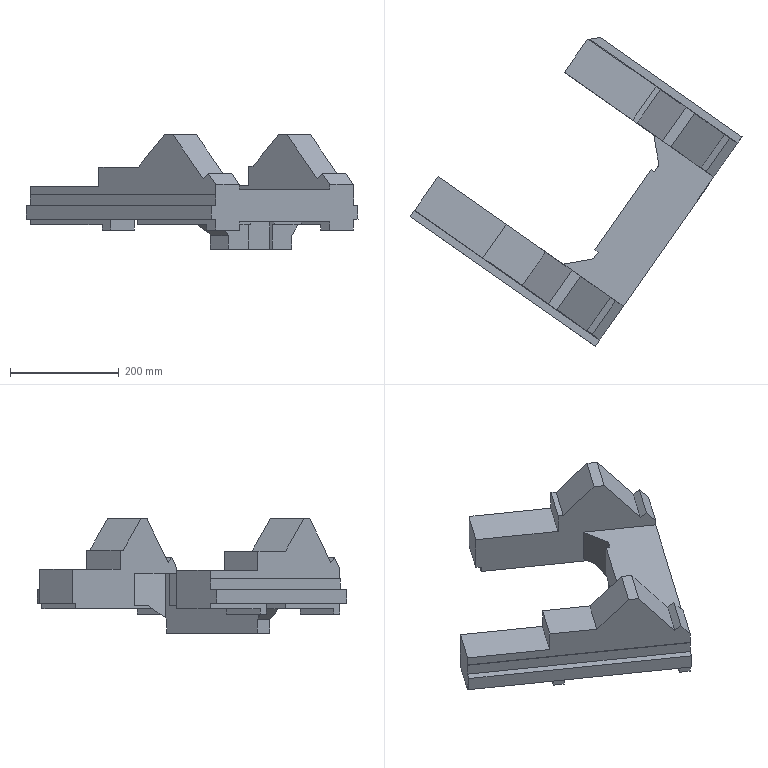Part | NX | features solid 2 | 1 solid | 74 faces | box 609.529 x 567.358 x 210 mm | volume 8240791 mm3 | plane 74